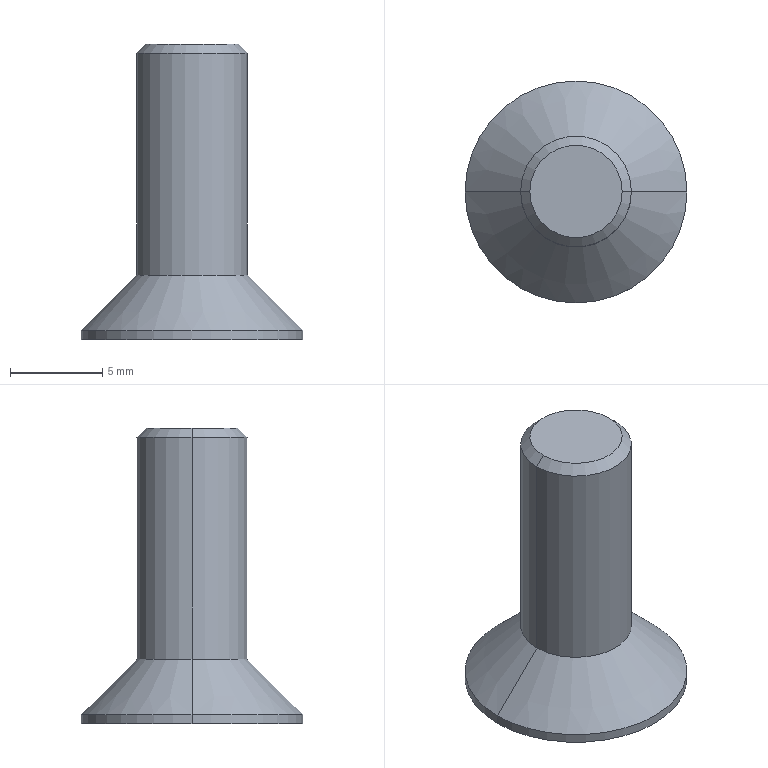Part | Creo | 1 solid | 17 faces | box 12 x 12 x 16 mm | volume 550.247 mm3 | plane 9 | cone 4 | cylinder 4 | commonest cylinder face diameters 6 x2 12 x2
STEP:
#1=CARTESIAN_POINT('',(0.,0.,0.));
#2=DIRECTION('',(0.,0.,1.));
#3=DIRECTION('',(1.,0.,0.));
#4=AXIS2_PLACEMENT_3D('',#1,#2,#3);
#5=CARTESIAN_POINT('',(62.,35.,-256.));
#6=VERTEX_POINT('',#5);
#7=CARTESIAN_POINT('',(68.,35.,-256.));
#8=VERTEX_POINT('',#7);
#9=CARTESIAN_POINT('',(65.,35.,-256.));
#10=DIRECTION('',(0.,0.,-1.));
#11=DIRECTION('',(-1.,0.,0.));
#12=AXIS2_PLACEMENT_3D('',#9,#10,#11);
#13=CIRCLE('',#12,3.);
#14=EDGE_CURVE('',#6,#8,#13,.T.);
#15=ORIENTED_EDGE('',*,*,#14,.F.);
#16=CARTESIAN_POINT('',(59.,35.,-259.));
#17=VERTEX_POINT('',#16);
#18=CARTESIAN_POINT('',(62.,35.,-256.));
#19=DIRECTION('',(-0.7071,0.,-0.7071));
#20=VECTOR('',#19,4.243);
#21=LINE('',#18,#20);
#22=EDGE_CURVE('',#6,#17,#21,.T.);
#23=ORIENTED_EDGE('',*,*,#22,.T.);
#24=CARTESIAN_POINT('',(71.,35.,-259.));
#25=VERTEX_POINT('',#24);
#26=CARTESIAN_POINT('',(65.,35.,-259.));
#27=DIRECTION('',(0.,0.,1.));
#28=DIRECTION('',(1.,0.,0.));
#29=AXIS2_PLACEMENT_3D('',#26,#27,#28);
#30=CIRCLE('',#29,6.);
#31=EDGE_CURVE('',#25,#17,#30,.T.);
#32=ORIENTED_EDGE('',*,*,#31,.F.);
#33=CARTESIAN_POINT('',(68.,35.,-256.));
#34=DIRECTION('',(0.7071,0.,-0.7071));
#35=VECTOR('',#34,4.243);
#36=LINE('',#33,#35);
#37=EDGE_CURVE('',#8,#25,#36,.T.);
#38=ORIENTED_EDGE('',*,*,#37,.F.);
#39=EDGE_LOOP('',(#15,#23,#32,#38));
#40=FACE_OUTER_BOUND('',#39,.F.);
#41=CARTESIAN_POINT('',(65.,35.,-257.5));
#42=DIRECTION('',(0.,0.,-1.));
#43=DIRECTION('',(-1.,0.,0.));
#44=AXIS2_PLACEMENT_3D('',#41,#42,#43);
#45=CONICAL_SURFACE('',#44,4.5,45.);
#46=ADVANCED_FACE('',(#40),#45,.T.);
#47=CARTESIAN_POINT('',(68.,35.,-244.));
#48=VERTEX_POINT('',#47);
#49=CARTESIAN_POINT('',(62.,35.,-244.));
#50=VERTEX_POINT('',#49);
#51=CARTESIAN_POINT('',(65.,35.,-244.));
#52=DIRECTION('',(0.,0.,1.));
#53=DIRECTION('',(1.,0.,0.));
#54=AXIS2_PLACEMENT_3D('',#51,#52,#53);
#55=CIRCLE('',#54,3.);
#56=EDGE_CURVE('',#48,#50,#55,.T.);
#57=ORIENTED_EDGE('',*,*,#56,.T.);
#58=CARTESIAN_POINT('',(62.,35.,-256.));
#59=DIRECTION('',(0.,0.,1.));
#60=VECTOR('',#59,12.);
#61=LINE('',#58,#60);
#62=EDGE_CURVE('',#6,#50,#61,.T.);
#63=ORIENTED_EDGE('',*,*,#62,.F.);
#64=ORIENTED_EDGE('',*,*,#14,.T.);
#65=CARTESIAN_POINT('',(68.,35.,-256.));
#66=DIRECTION('',(0.,0.,1.));
#67=VECTOR('',#66,12.);
#68=LINE('',#65,#67);
#69=EDGE_CURVE('',#8,#48,#68,.T.);
#70=ORIENTED_EDGE('',*,*,#69,.T.);
#71=EDGE_LOOP('',(#57,#63,#64,#70));
#72=FACE_OUTER_BOUND('',#71,.F.);
#73=CARTESIAN_POINT('',(65.,35.,-255.5));
#74=DIRECTION('',(0.,0.,1.));
#75=DIRECTION('',(1.,0.,0.));
#76=AXIS2_PLACEMENT_3D('',#73,#74,#75);
#77=CYLINDRICAL_SURFACE('',#76,3.);
#78=ADVANCED_FACE('',(#72),#77,.T.);
#79=ORIENTED_EDGE('',*,*,#56,.F.);
#80=CARTESIAN_POINT('',(67.5,35.,-243.5));
#81=VERTEX_POINT('',#80);
#82=CARTESIAN_POINT('',(67.5,35.,-243.5));
#83=DIRECTION('',(0.7071,0.,-0.7071));
#84=VECTOR('',#83,0.7071);
#85=LINE('',#82,#84);
#86=EDGE_CURVE('',#81,#48,#85,.T.);
#87=ORIENTED_EDGE('',*,*,#86,.F.);
#88=CARTESIAN_POINT('',(62.5,35.,-243.5));
#89=VERTEX_POINT('',#88);
#90=CARTESIAN_POINT('',(65.,35.,-243.5));
#91=DIRECTION('',(0.,0.,1.));
#92=DIRECTION('',(1.,0.,0.));
#93=AXIS2_PLACEMENT_3D('',#90,#91,#92);
#94=CIRCLE('',#93,2.5);
#95=EDGE_CURVE('',#81,#89,#94,.T.);
#96=ORIENTED_EDGE('',*,*,#95,.T.);
#97=CARTESIAN_POINT('',(62.5,35.,-243.5));
#98=DIRECTION('',(-0.7071,0.,-0.7071));
#99=VECTOR('',#98,0.7071);
#100=LINE('',#97,#99);
#101=EDGE_CURVE('',#89,#50,#100,.T.);
#102=ORIENTED_EDGE('',*,*,#101,.T.);
#103=EDGE_LOOP('',(#79,#87,#96,#102));
#104=FACE_OUTER_BOUND('',#103,.F.);
#105=CARTESIAN_POINT('',(65.,35.,-243.75));
#106=DIRECTION('',(0.,0.,-1.));
#107=DIRECTION('',(-1.,0.,0.));
#108=AXIS2_PLACEMENT_3D('',#105,#106,#107);
#109=CONICAL_SURFACE('',#108,2.75,45.);
#110=ADVANCED_FACE('',(#104),#109,.T.);
#111=CARTESIAN_POINT('',(65.,35.,-244.));
#112=DIRECTION('',(0.,0.,1.));
#113=DIRECTION('',(-1.,0.,0.));
#114=AXIS2_PLACEMENT_3D('',#111,#112,#113);
#115=CIRCLE('',#114,3.);
#116=EDGE_CURVE('',#50,#48,#115,.T.);
#117=ORIENTED_EDGE('',*,*,#116,.F.);
#118=ORIENTED_EDGE('',*,*,#101,.F.);
#119=CARTESIAN_POINT('',(65.,35.,-243.5));
#120=DIRECTION('',(0.,0.,1.));
#121=DIRECTION('',(-1.,0.,0.));
#122=AXIS2_PLACEMENT_3D('',#119,#120,#121);
#123=CIRCLE('',#122,2.5);
#124=EDGE_CURVE('',#89,#81,#123,.T.);
#125=ORIENTED_EDGE('',*,*,#124,.T.);
#126=ORIENTED_EDGE('',*,*,#86,.T.);
#127=EDGE_LOOP('',(#117,#118,#125,#126));
#128=FACE_OUTER_BOUND('',#127,.F.);
#129=CARTESIAN_POINT('',(65.,35.,-243.75));
#130=DIRECTION('',(0.,0.,-1.));
#131=DIRECTION('',(-1.,0.,0.));
#132=AXIS2_PLACEMENT_3D('',#129,#130,#131);
#133=CONICAL_SURFACE('',#132,2.75,45.);
#134=ADVANCED_FACE('',(#128),#133,.T.);
#135=ORIENTED_EDGE('',*,*,#116,.T.);
#136=ORIENTED_EDGE('',*,*,#69,.F.);
#137=CARTESIAN_POINT('',(65.,35.,-256.));
#138=DIRECTION('',(0.,0.,-1.));
#139=DIRECTION('',(1.,0.,0.));
#140=AXIS2_PLACEMENT_3D('',#137,#138,#139);
#141=CIRCLE('',#140,3.);
#142=EDGE_CURVE('',#8,#6,#141,.T.);
#143=ORIENTED_EDGE('',*,*,#142,.T.);
#144=ORIENTED_EDGE('',*,*,#62,.T.);
#145=EDGE_LOOP('',(#135,#136,#143,#144));
#146=FACE_OUTER_BOUND('',#145,.F.);
#147=CARTESIAN_POINT('',(65.,35.,-255.5));
#148=DIRECTION('',(0.,0.,1.));
#149=DIRECTION('',(1.,0.,0.));
#150=AXIS2_PLACEMENT_3D('',#147,#148,#149);
#151=CYLINDRICAL_SURFACE('',#150,3.);
#152=ADVANCED_FACE('',(#146),#151,.T.);
#153=ORIENTED_EDGE('',*,*,#142,.F.);
#154=ORIENTED_EDGE('',*,*,#37,.T.);
#155=CARTESIAN_POINT('',(65.,35.,-259.));
#156=DIRECTION('',(0.,0.,1.));
#157=DIRECTION('',(-1.,0.,0.));
#158=AXIS2_PLACEMENT_3D('',#155,#156,#157);
#159=CIRCLE('',#158,6.);
#160=EDGE_CURVE('',#17,#25,#159,.T.);
#161=ORIENTED_EDGE('',*,*,#160,.F.);
#162=ORIENTED_EDGE('',*,*,#22,.F.);
#163=EDGE_LOOP('',(#153,#154,#161,#162));
#164=FACE_OUTER_BOUND('',#163,.F.);
#165=CARTESIAN_POINT('',(65.,35.,-257.5));
#166=DIRECTION('',(0.,0.,-1.));
#167=DIRECTION('',(-1.,0.,0.));
#168=AXIS2_PLACEMENT_3D('',#165,#166,#167);
#169=CONICAL_SURFACE('',#168,4.5,45.);
#170=ADVANCED_FACE('',(#164),#169,.T.);
#171=ORIENTED_EDGE('',*,*,#160,.T.);
#172=CARTESIAN_POINT('',(71.,35.,-259.5));
#173=VERTEX_POINT('',#172);
#174=CARTESIAN_POINT('',(71.,35.,-259.));
#175=DIRECTION('',(0.,0.,-1.));
#176=VECTOR('',#175,0.5);
#177=LINE('',#174,#176);
#178=EDGE_CURVE('',#25,#173,#177,.T.);
#179=ORIENTED_EDGE('',*,*,#178,.T.);
#180=CARTESIAN_POINT('',(59.,35.,-259.5));
#181=VERTEX_POINT('',#180);
#182=CARTESIAN_POINT('',(65.,35.,-259.5));
#183=DIRECTION('',(0.,0.,-1.));
#184=DIRECTION('',(1.,0.,0.));
#185=AXIS2_PLACEMENT_3D('',#182,#183,#184);
#186=CIRCLE('',#185,6.);
#187=EDGE_CURVE('',#173,#181,#186,.T.);
#188=ORIENTED_EDGE('',*,*,#187,.T.);
#189=CARTESIAN_POINT('',(59.,35.,-259.));
#190=DIRECTION('',(0.,0.,-1.));
#191=VECTOR('',#190,0.5);
#192=LINE('',#189,#191);
#193=EDGE_CURVE('',#17,#181,#192,.T.);
#194=ORIENTED_EDGE('',*,*,#193,.F.);
#195=EDGE_LOOP('',(#171,#179,#188,#194));
#196=FACE_OUTER_BOUND('',#195,.F.);
#197=CARTESIAN_POINT('',(65.,35.,-257.5));
#198=DIRECTION('',(0.,0.,-1.));
#199=DIRECTION('',(-1.,0.,0.));
#200=AXIS2_PLACEMENT_3D('',#197,#198,#199);
#201=CYLINDRICAL_SURFACE('',#200,6.);
#202=ADVANCED_FACE('',(#196),#201,.T.);
#203=ORIENTED_EDGE('',*,*,#31,.T.);
#204=ORIENTED_EDGE('',*,*,#193,.T.);
#205=CARTESIAN_POINT('',(65.,35.,-259.5));
#206=DIRECTION('',(0.,0.,-1.));
#207=DIRECTION('',(-1.,0.,0.));
#208=AXIS2_PLACEMENT_3D('',#205,#206,#207);
#209=CIRCLE('',#208,6.);
#210=EDGE_CURVE('',#181,#173,#209,.T.);
#211=ORIENTED_EDGE('',*,*,#210,.T.);
#212=ORIENTED_EDGE('',*,*,#178,.F.);
#213=EDGE_LOOP('',(#203,#204,#211,#212));
#214=FACE_OUTER_BOUND('',#213,.F.);
#215=CARTESIAN_POINT('',(65.,35.,-257.5));
#216=DIRECTION('',(0.,0.,-1.));
#217=DIRECTION('',(-1.,0.,0.));
#218=AXIS2_PLACEMENT_3D('',#215,#216,#217);
#219=CYLINDRICAL_SURFACE('',#218,6.);
#220=ADVANCED_FACE('',(#214),#219,.T.);
#221=ORIENTED_EDGE('',*,*,#187,.F.);
#222=ORIENTED_EDGE('',*,*,#210,.F.);
#223=EDGE_LOOP('',(#221,#222));
#224=FACE_OUTER_BOUND('',#223,.F.);
#225=CARTESIAN_POINT('',(67.,33.845,-259.5));
#226=VERTEX_POINT('',#225);
#227=CARTESIAN_POINT('',(67.,36.155,-259.5));
#228=VERTEX_POINT('',#227);
#229=CARTESIAN_POINT('',(67.,33.845,-259.5));
#230=DIRECTION('',(0.,1.,0.));
#231=VECTOR('',#230,2.309);
#232=LINE('',#229,#231);
#233=EDGE_CURVE('',#226,#228,#232,.T.);
#234=ORIENTED_EDGE('',*,*,#233,.F.);
#235=CARTESIAN_POINT('',(65.,32.691,-259.5));
#236=VERTEX_POINT('',#235);
#237=CARTESIAN_POINT('',(65.,32.691,-259.5));
#238=DIRECTION('',(0.866,0.5,0.));
#239=VECTOR('',#238,2.309);
#240=LINE('',#237,#239);
#241=EDGE_CURVE('',#236,#226,#240,.T.);
#242=ORIENTED_EDGE('',*,*,#241,.F.);
#243=CARTESIAN_POINT('',(63.,33.845,-259.5));
#244=VERTEX_POINT('',#243);
#245=CARTESIAN_POINT('',(63.,33.845,-259.5));
#246=DIRECTION('',(0.866,-0.5,0.));
#247=VECTOR('',#246,2.309);
#248=LINE('',#245,#247);
#249=EDGE_CURVE('',#244,#236,#248,.T.);
#250=ORIENTED_EDGE('',*,*,#249,.F.);
#251=CARTESIAN_POINT('',(63.,36.155,-259.5));
#252=VERTEX_POINT('',#251);
#253=CARTESIAN_POINT('',(63.,36.155,-259.5));
#254=DIRECTION('',(0.,-1.,0.));
#255=VECTOR('',#254,2.309);
#256=LINE('',#253,#255);
#257=EDGE_CURVE('',#252,#244,#256,.T.);
#258=ORIENTED_EDGE('',*,*,#257,.F.);
#259=CARTESIAN_POINT('',(65.,37.309,-259.5));
#260=VERTEX_POINT('',#259);
#261=CARTESIAN_POINT('',(65.,37.309,-259.5));
#262=DIRECTION('',(-0.866,-0.5,0.));
#263=VECTOR('',#262,2.309);
#264=LINE('',#261,#263);
#265=EDGE_CURVE('',#260,#252,#264,.T.);
#266=ORIENTED_EDGE('',*,*,#265,.F.);
#267=CARTESIAN_POINT('',(67.,36.155,-259.5));
#268=DIRECTION('',(-0.866,0.5,0.));
#269=VECTOR('',#268,2.309);
#270=LINE('',#267,#269);
#271=EDGE_CURVE('',#228,#260,#270,.T.);
#272=ORIENTED_EDGE('',*,*,#271,.F.);
#273=EDGE_LOOP('',(#234,#242,#250,#258,#266,#272));
#274=FACE_BOUND('',#273,.F.);
#275=CARTESIAN_POINT('',(65.,35.,-259.5));
#276=DIRECTION('',(0.,0.,1.));
#277=DIRECTION('',(1.,0.,0.));
#278=AXIS2_PLACEMENT_3D('',#275,#276,#277);
#279=PLANE('',#278);
#280=ADVANCED_FACE('',(#224,#274),#279,.F.);
#281=ORIENTED_EDGE('',*,*,#233,.T.);
#282=CARTESIAN_POINT('',(67.,36.155,-255.5));
#283=VERTEX_POINT('',#282);
#284=CARTESIAN_POINT('',(67.,36.155,-255.5));
#285=DIRECTION('',(0.,0.,-1.));
#286=VECTOR('',#285,4.);
#287=LINE('',#284,#286);
#288=EDGE_CURVE('',#283,#228,#287,.T.);
#289=ORIENTED_EDGE('',*,*,#288,.F.);
#290=CARTESIAN_POINT('',(67.,33.845,-255.5));
#291=VERTEX_POINT('',#290);
#292=CARTESIAN_POINT('',(67.,36.155,-255.5));
#293=DIRECTION('',(0.,-1.,0.));
#294=VECTOR('',#293,2.309);
#295=LINE('',#292,#294);
#296=EDGE_CURVE('',#283,#291,#295,.T.);
#297=ORIENTED_EDGE('',*,*,#296,.T.);
#298=CARTESIAN_POINT('',(67.,33.845,-255.5));
#299=DIRECTION('',(0.,0.,-1.));
#300=VECTOR('',#299,4.);
#301=LINE('',#298,#300);
#302=EDGE_CURVE('',#291,#226,#301,.T.);
#303=ORIENTED_EDGE('',*,*,#302,.T.);
#304=EDGE_LOOP('',(#281,#289,#297,#303));
#305=FACE_OUTER_BOUND('',#304,.F.);
#306=CARTESIAN_POINT('',(67.,36.155,-255.5));
#307=DIRECTION('',(1.,0.,0.));
#308=DIRECTION('',(0.,-1.,0.));
#309=AXIS2_PLACEMENT_3D('',#306,#307,#308);
#310=PLANE('',#309);
#311=ADVANCED_FACE('',(#305),#310,.F.);
#312=ORIENTED_EDGE('',*,*,#271,.T.);
#313=CARTESIAN_POINT('',(65.,37.309,-255.5));
#314=VERTEX_POINT('',#313);
#315=CARTESIAN_POINT('',(65.,37.309,-255.5));
#316=DIRECTION('',(0.,0.,-1.));
#317=VECTOR('',#316,4.);
#318=LINE('',#315,#317);
#319=EDGE_CURVE('',#314,#260,#318,.T.);
#320=ORIENTED_EDGE('',*,*,#319,.F.);
#321=CARTESIAN_POINT('',(65.,37.309,-255.5));
#322=DIRECTION('',(0.866,-0.5,0.));
#323=VECTOR('',#322,2.309);
#324=LINE('',#321,#323);
#325=EDGE_CURVE('',#314,#283,#324,.T.);
#326=ORIENTED_EDGE('',*,*,#325,.T.);
#327=ORIENTED_EDGE('',*,*,#288,.T.);
#328=EDGE_LOOP('',(#312,#320,#326,#327));
#329=FACE_OUTER_BOUND('',#328,.F.);
#330=CARTESIAN_POINT('',(65.,37.309,-255.5));
#331=DIRECTION('',(0.5,0.866,0.));
#332=DIRECTION('',(0.866,-0.5,0.));
#333=AXIS2_PLACEMENT_3D('',#330,#331,#332);
#334=PLANE('',#333);
#335=ADVANCED_FACE('',(#329),#334,.F.);
#336=ORIENTED_EDGE('',*,*,#265,.T.);
#337=CARTESIAN_POINT('',(63.,36.155,-255.5));
#338=VERTEX_POINT('',#337);
#339=CARTESIAN_POINT('',(63.,36.155,-255.5));
#340=DIRECTION('',(0.,0.,-1.));
#341=VECTOR('',#340,4.);
#342=LINE('',#339,#341);
#343=EDGE_CURVE('',#338,#252,#342,.T.);
#344=ORIENTED_EDGE('',*,*,#343,.F.);
#345=CARTESIAN_POINT('',(63.,36.155,-255.5));
#346=DIRECTION('',(0.866,0.5,0.));
#347=VECTOR('',#346,2.309);
#348=LINE('',#345,#347);
#349=EDGE_CURVE('',#338,#314,#348,.T.);
#350=ORIENTED_EDGE('',*,*,#349,.T.);
#351=ORIENTED_EDGE('',*,*,#319,.T.);
#352=EDGE_LOOP('',(#336,#344,#350,#351));
#353=FACE_OUTER_BOUND('',#352,.F.);
#354=CARTESIAN_POINT('',(63.,36.155,-255.5));
#355=DIRECTION('',(-0.5,0.866,0.));
#356=DIRECTION('',(0.866,0.5,0.));
#357=AXIS2_PLACEMENT_3D('',#354,#355,#356);
#358=PLANE('',#357);
#359=ADVANCED_FACE('',(#353),#358,.F.);
#360=ORIENTED_EDGE('',*,*,#257,.T.);
#361=CARTESIAN_POINT('',(63.,33.845,-255.5));
#362=VERTEX_POINT('',#361);
#363=CARTESIAN_POINT('',(63.,33.845,-255.5));
#364=DIRECTION('',(0.,0.,-1.));
#365=VECTOR('',#364,4.);
#366=LINE('',#363,#365);
#367=EDGE_CURVE('',#362,#244,#366,.T.);
#368=ORIENTED_EDGE('',*,*,#367,.F.);
#369=CARTESIAN_POINT('',(63.,33.845,-255.5));
#370=DIRECTION('',(0.,1.,0.));
#371=VECTOR('',#370,2.309);
#372=LINE('',#369,#371);
#373=EDGE_CURVE('',#362,#338,#372,.T.);
#374=ORIENTED_EDGE('',*,*,#373,.T.);
#375=ORIENTED_EDGE('',*,*,#343,.T.);
#376=EDGE_LOOP('',(#360,#368,#374,#375));
#377=FACE_OUTER_BOUND('',#376,.F.);
#378=CARTESIAN_POINT('',(63.,33.845,-255.5));
#379=DIRECTION('',(-1.,0.,0.));
#380=DIRECTION('',(0.,0.,1.));
#381=AXIS2_PLACEMENT_3D('',#378,#379,#380);
#382=PLANE('',#381);
#383=ADVANCED_FACE('',(#377),#382,.F.);
#384=ORIENTED_EDGE('',*,*,#249,.T.);
#385=CARTESIAN_POINT('',(65.,32.691,-255.5));
#386=VERTEX_POINT('',#385);
#387=CARTESIAN_POINT('',(65.,32.691,-255.5));
#388=DIRECTION('',(0.,0.,-1.));
#389=VECTOR('',#388,4.);
#390=LINE('',#387,#389);
#391=EDGE_CURVE('',#386,#236,#390,.T.);
#392=ORIENTED_EDGE('',*,*,#391,.F.);
#393=CARTESIAN_POINT('',(65.,32.691,-255.5));
#394=DIRECTION('',(-0.866,0.5,0.));
#395=VECTOR('',#394,2.309);
#396=LINE('',#393,#395);
#397=EDGE_CURVE('',#386,#362,#396,.T.);
#398=ORIENTED_EDGE('',*,*,#397,.T.);
#399=ORIENTED_EDGE('',*,*,#367,.T.);
#400=EDGE_LOOP('',(#384,#392,#398,#399));
#401=FACE_OUTER_BOUND('',#400,.F.);
#402=CARTESIAN_POINT('',(65.,32.691,-255.5));
#403=DIRECTION('',(-0.5,-0.866,0.));
#404=DIRECTION('',(-0.866,0.5,0.));
#405=AXIS2_PLACEMENT_3D('',#402,#403,#404);
#406=PLANE('',#405);
#407=ADVANCED_FACE('',(#401),#406,.F.);
#408=ORIENTED_EDGE('',*,*,#241,.T.);
#409=ORIENTED_EDGE('',*,*,#302,.F.);
#410=CARTESIAN_POINT('',(67.,33.845,-255.5));
#411=DIRECTION('',(-0.866,-0.5,0.));
#412=VECTOR('',#411,2.309);
#413=LINE('',#410,#412);
#414=EDGE_CURVE('',#291,#386,#413,.T.);
#415=ORIENTED_EDGE('',*,*,#414,.T.);
#416=ORIENTED_EDGE('',*,*,#391,.T.);
#417=EDGE_LOOP('',(#408,#409,#415,#416));
#418=FACE_OUTER_BOUND('',#417,.F.);
#419=CARTESIAN_POINT('',(67.,33.845,-255.5));
#420=DIRECTION('',(0.5,-0.866,0.));
#421=DIRECTION('',(-0.866,-0.5,0.));
#422=AXIS2_PLACEMENT_3D('',#419,#420,#421);
#423=PLANE('',#422);
#424=ADVANCED_FACE('',(#418),#423,.F.);
#425=ORIENTED_EDGE('',*,*,#296,.F.);
#426=ORIENTED_EDGE('',*,*,#325,.F.);
#427=ORIENTED_EDGE('',*,*,#349,.F.);
#428=ORIENTED_EDGE('',*,*,#373,.F.);
#429=ORIENTED_EDGE('',*,*,#397,.F.);
#430=ORIENTED_EDGE('',*,*,#414,.F.);
#431=EDGE_LOOP('',(#425,#426,#427,#428,#429,#430));
#432=FACE_OUTER_BOUND('',#431,.F.);
#433=CARTESIAN_POINT('',(65.,35.,-255.5));
#434=DIRECTION('',(0.,0.,-1.));
#435=DIRECTION('',(-1.,0.,0.));
#436=AXIS2_PLACEMENT_3D('',#433,#434,#435);
#437=PLANE('',#436);
#438=ADVANCED_FACE('',(#432),#437,.T.);
#439=ORIENTED_EDGE('',*,*,#124,.F.);
#440=ORIENTED_EDGE('',*,*,#95,.F.);
#441=EDGE_LOOP('',(#439,#440));
#442=FACE_OUTER_BOUND('',#441,.F.);
#443=CARTESIAN_POINT('',(65.,32.,-243.5));
#444=DIRECTION('',(0.,0.,-1.));
#445=DIRECTION('',(-1.,0.,0.));
#446=AXIS2_PLACEMENT_3D('',#443,#444,#445);
#447=PLANE('',#446);
#448=ADVANCED_FACE('',(#442),#447,.F.);
#449=CLOSED_SHELL('',(#46,#78,#110,#134,#152,#170,#202,#220,#280,#311,#335,#359,#383,#407,#424,#438,#448));
#450=MANIFOLD_SOLID_BREP('',#449);
#451=(LENGTH_UNIT()NAMED_UNIT(*)SI_UNIT(.MILLI.,.METRE.));
#452=UNCERTAINTY_MEASURE_WITH_UNIT(LENGTH_MEASURE(0.002332),#451,'','');
#453=(NAMED_UNIT(*)PLANE_ANGLE_UNIT()SI_UNIT($,.RADIAN.));
#454=PLANE_ANGLE_MEASURE_WITH_UNIT(PLANE_ANGLE_MEASURE(0.01745),#453);
#455=(CONVERSION_BASED_UNIT('DEGREE',#454)NAMED_UNIT(*)PLANE_ANGLE_UNIT());
#456=(NAMED_UNIT(*)SI_UNIT($,.STERADIAN.)SOLID_ANGLE_UNIT());
#457=(GEOMETRIC_REPRESENTATION_CONTEXT(3)GLOBAL_UNCERTAINTY_ASSIGNED_CONTEXT((#452))GLOBAL_UNIT_ASSIGNED_CONTEXT((#451,#455,#456))REPRESENTATION_CONTEXT('',''));
#458=ADVANCED_BREP_SHAPE_REPRESENTATION('',(#4,#450),#457);